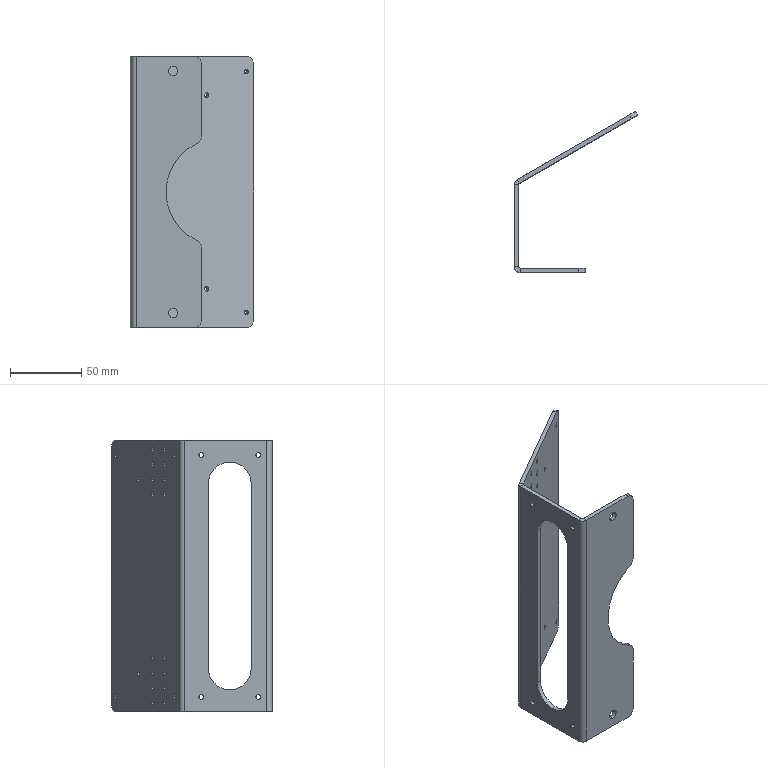Part | STEP file | 1 solid | 90 faces | box 86.5 x 113.075 x 190 mm | volume 98833 mm3 | cylinder 69 | plane 21 | commonest cylinder face diameters 3.3 x52 10 x6 6.5 x4 2 x2 8 x2 30 x2